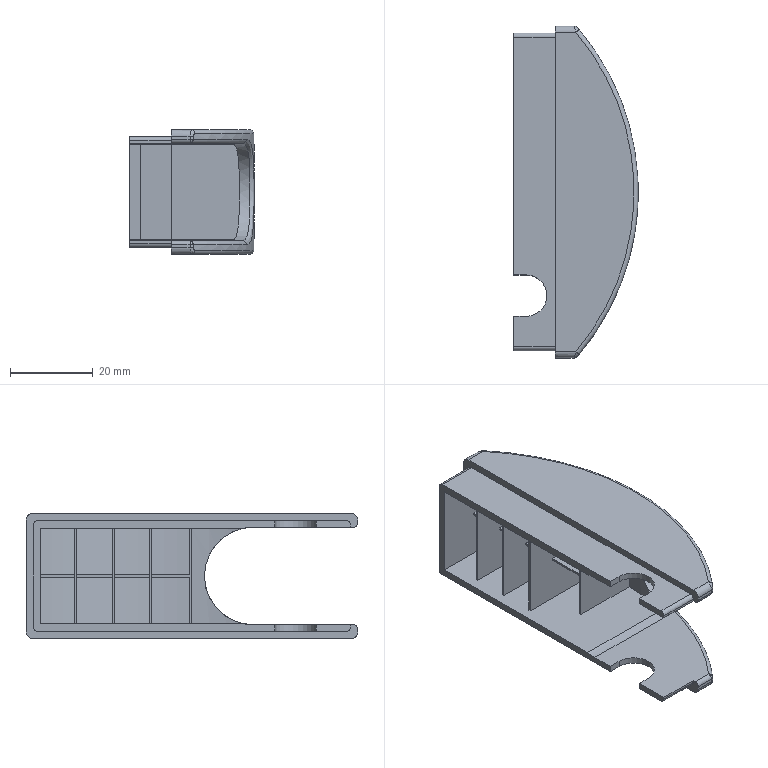Part | STEP file | 7100102W | 1 solid | 94 faces | box 30 x 80 x 30 mm | volume 16145 mm3 | plane 51 | cylinder 32 | spline 5 | torus 4 | sphere 2 | commonest cylinder face diameters 2 x9 114.667 x9 3 x4 6 x4 121.667 x3 10 x2